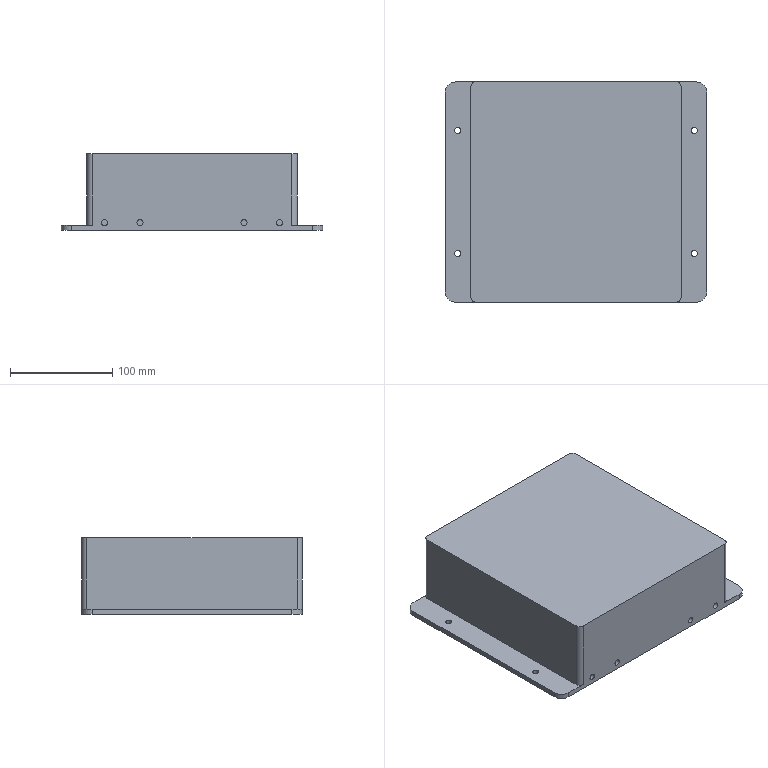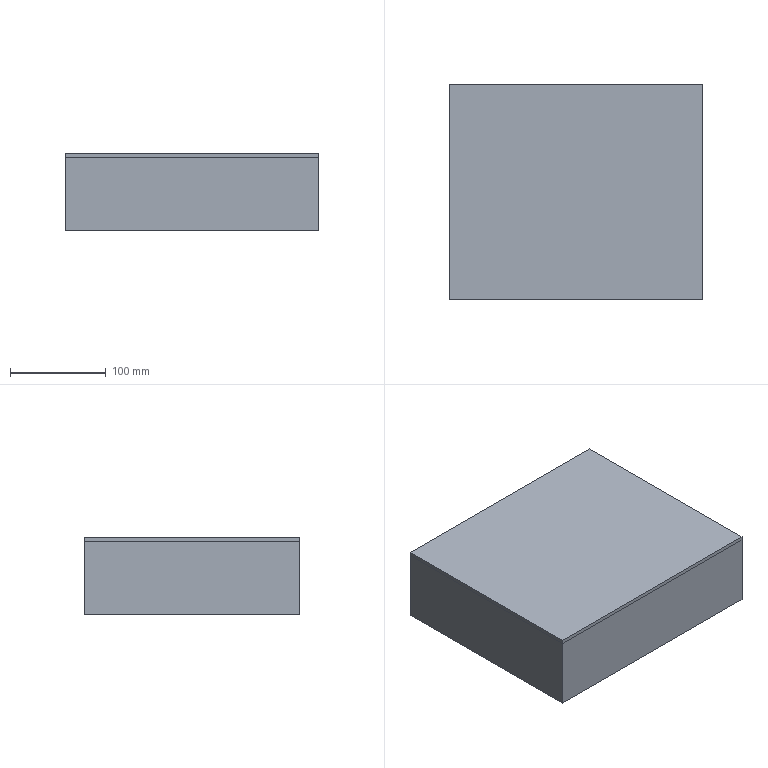CAM job | NX | 3+2 milling, drilling | part box 255 x 215 x 75 mm | stock box 265 x 225 x 80 mm
Tools:
number,name,description,diameter,corner_radius,flute_length,length,flutes
19,D80,Milling Tool-5 Parameters,80.0,0.0,50.0,75.0,2
14,D10JING,Milling Tool-5 Parameters,10.0,0.0,50.0,75.0,2
1,D6A45,Milling Tool-5 Parameters,6.0,0.0,50.0,75.0,2
16,6.0ZT,Drilling Tool,6.0,0.0,35.0,50.0,2
12,D6,Milling Tool-5 Parameters,6.0,0.0,50.0,75.0,2
17,R3,Milling Tool-5 Parameters,6.0,3.0,50.0,75.0,2
18,D16,Milling Tool-5 Parameters,16.0,0.0,50.0,75.0,2
Operations:
program,operation,operation_type,tool,method,geometry_group,spindle_rpm,surface_speed,feed_per_tooth,feed_cut,feed_plunge,cut_length_mm,path_length_mm,cut_time_min,machine_time_min
1,FLOOR_WALL,VolumeBased25DMillingOperation,D80,METHOD,A,6500.0,1633.0,0.1154,1500.0,100.0,1929.997,1983.997,1.287,1.292
1,ZLEVEL_PROFILE_COPY_1,ZLevelMilling,D16,METHOD,A,8000.0,402.0,0.1875,3000.0,1000.0,74051.352,74183.352,24.716,24.729
1,FLOOR_WALL_1,VolumeBased25DMillingOperation,D16,METHOD,A,9500.0,298.0,0.1316,2500.0,1000.0,136450.766,138544.008,54.921,55.131
1,ZLEVEL_PROFILE_COPY_1_COPY,ZLevelMilling,D10JING,METHOD,A,9500.0,298.0,0.0632,1200.0,1000.0,4819.031,5562.888,4.021,4.095
1,ZLEVEL_PROFILE_COPY_1_COPY_COPY,ZLevelMilling,D10JING,METHOD,A,9500.0,298.0,0.0632,1200.0,1000.0,2462.236,5884.341,2.062,2.404
1,FLOOR_WALL_1_COPY,VolumeBased25DMillingOperation,D10JING,METHOD,A,9500.0,298.0,0.0632,1200.0,1000.0,3222.765,4381.961,2.724,2.84
1,PLANAR_MILL_COPY_COPY_COPY_COPY,PlanarMilling,D6A45,METHOD,A,9500.0,179.0,0.0658,1250.0,100.0,846.923,906.923,0.6775,0.6835
2,FLOOR_WALL_COPY,VolumeBased25DMillingOperation,D80,METHOD,B,6500.0,1633.0,0.1154,1500.0,100.0,9649.985,11502.229,6.433,6.619
2,DRILLING,Operation,D6A45,METHOD,B,5000.0,94.0,0.035,350.0,0.0,16.0,572.095,0.0457,0.1013
2,DRILLING_COPY,Operation,6.0ZT,METHOD,B,2000.0,37.0,0.0625,250.0,0.0,45.21,630.515,0.1808,0.2394
2,FLOOR_WALL_1_COPY_1,VolumeBased25DMillingOperation,D16,METHOD,B,9500.0,477.0,0.1316,2500.0,1000.0,282214.873,288308.765,114.891,115.501
2,ZLEVEL_PROFILE_COPY,ZLevelMilling,D10JING,METHOD,B,9500.0,179.0,0.0658,1250.0,100.0,7760.109,11105.303,6.208,6.543
2,FLOOR_WALL_1_COPY_COPY,VolumeBased25DMillingOperation,D10JING,METHOD,B,9500.0,298.0,0.0632,1200.0,1000.0,8311.191,8509.191,6.926,6.946
2,ZLEVEL_PROFILE_COPY_1_COPY_COPY_COPY,ZLevelMilling,D10JING,METHOD,B,9500.0,298.0,0.0632,1200.0,1000.0,3847.652,4561.509,3.211,3.283
2,ZLEVEL_PROFILE,ZLevelMilling,D6,METHOD,B,9500.0,179.0,0.0658,1250.0,100.0,606.082,2134.062,0.4849,0.6377
2,FIXED_CONTOUR,SurfaceContour,R3,METHOD,B,9500.0,179.0,0.1053,2000.0,100.0,239.339,295.739,0.1197,0.1253
2,PLANAR_MILL_COPY_COPY_COPY_COPY_COPY,PlanarMilling,D6A45,METHOD,B,9500.0,179.0,0.0658,1250.0,100.0,1778.729,2574.55,1.423,1.503
3,DRILLING_COPY_1,Operation,D6A45,METHOD,C,5000.0,94.0,0.035,350.0,0.0,16.0,271.805,0.0457,0.0713
3,DRILLING_COPY_COPY,Operation,6.0ZT,METHOD,C,2000.0,37.0,0.0625,250.0,0.0,45.21,330.225,0.1808,0.2093